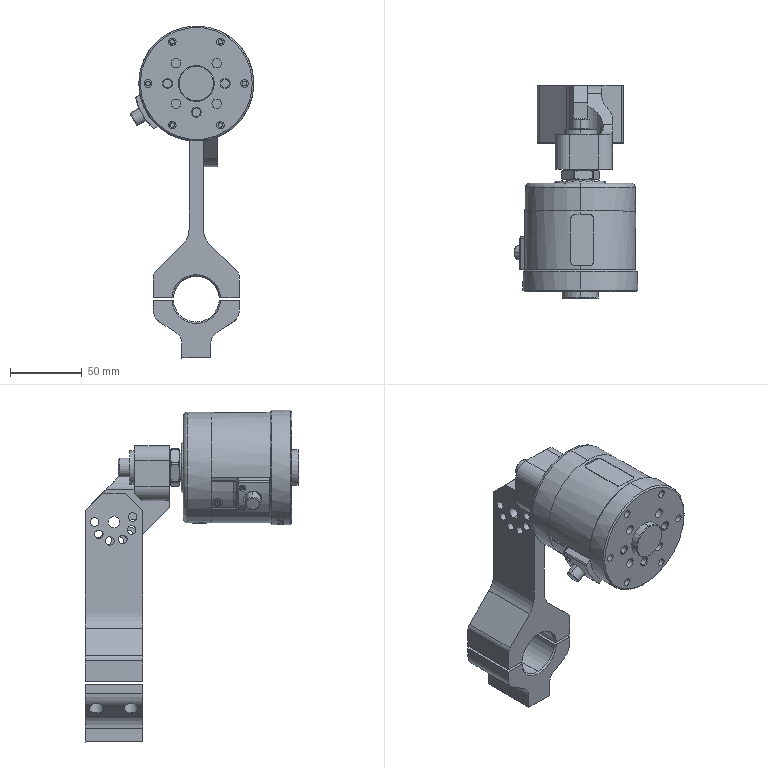Part | STEP file | 780.0885.0+780.H027.0+780.0512.1+780.0029 | 12 solids | 740 faces | box 85.965 x 148.6 x 231 mm | volume 538437 mm3 | cylinder 283 | plane 217 | cone 138 | spline 92 | torus 10 | commonest cylinder face diameters 6 x55 4 x17 5 x16 20 x14 3.3 x12 5.3 x12